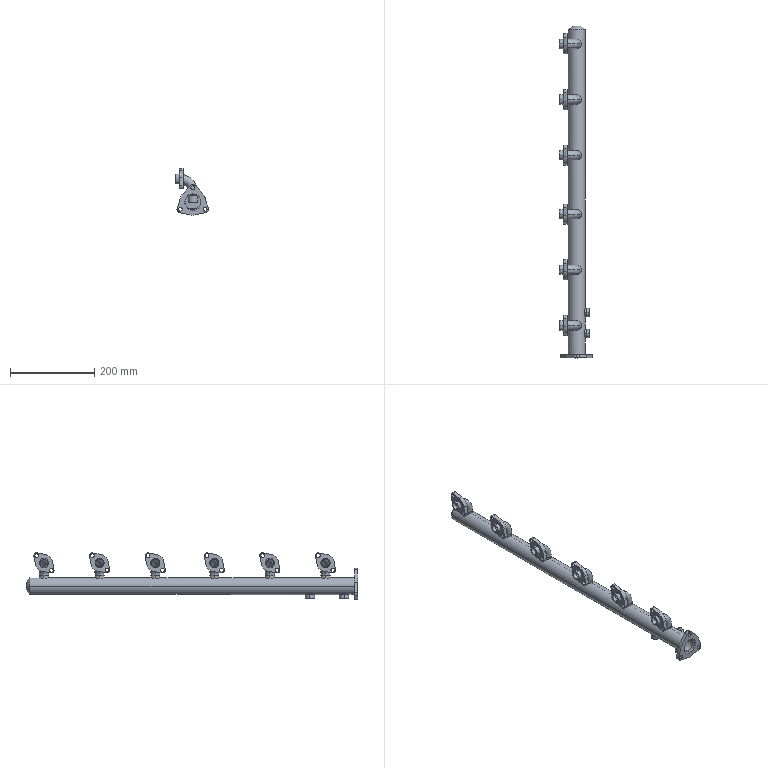Part | SolidWorks | features BaseBody 12 | 12 solids | 494 faces | box 78.445 x 787.626 x 109.824 mm | volume 305348 mm3 | cylinder 355 | plane 99 | torus 26 | spline 12 | cone 2 | commonest cylinder face diameters 14 x74 22 x60 18 x48 15 x42 9 x30 12 x30